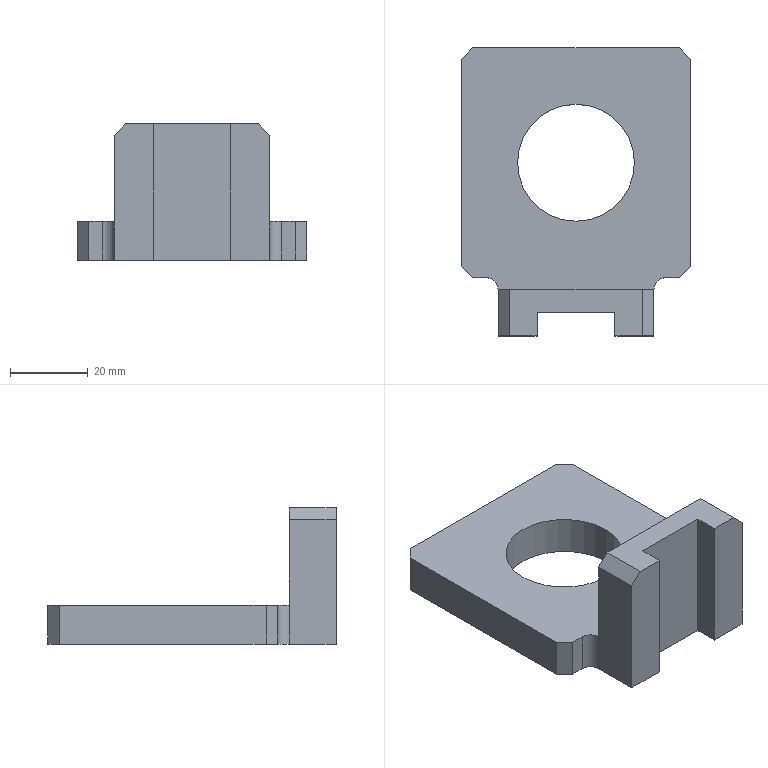Part | STEP file | PN_0015 | 1 solid | 26 faces | box 59 x 74 x 35 mm | volume 41292 mm3 | plane 22 | cylinder 4 | commonest cylinder face diameters 6 x2 30 x2